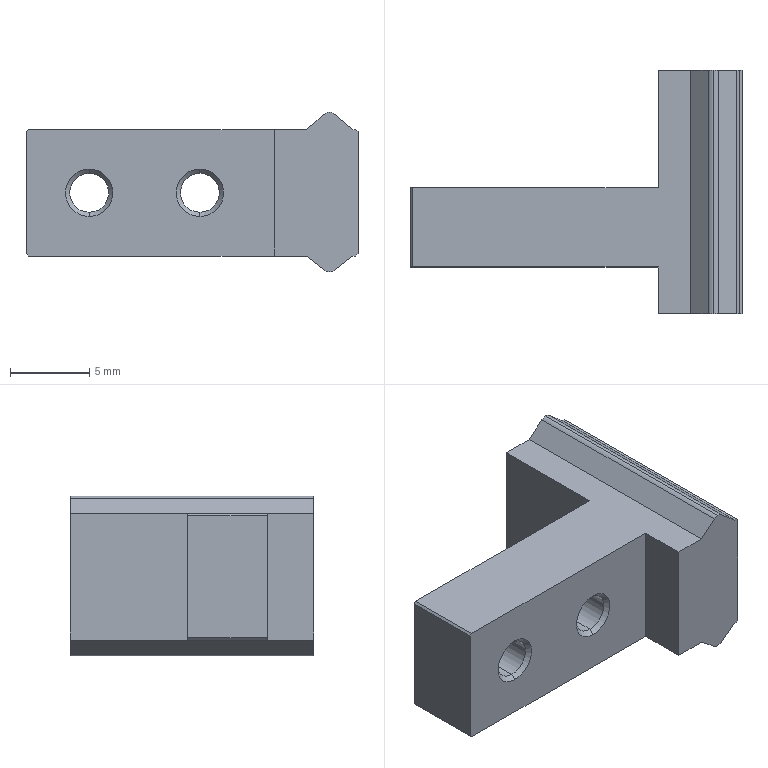Part | SolidWorks | features BaseBody 1 | 1 solid | 35 faces | box 21 x 15.4 x 10.1 mm | volume 1286 mm3 | plane 20 | cone 8 | cylinder 7 | commonest cylinder face diameters 2.459 x4 1 x3
STEP:
#1=CARTESIAN_POINT('',(-48.3,-0.01,5.1));
#2=VERTEX_POINT('',#1);
#3=CARTESIAN_POINT('',(-47.977,-0.01,4.981));
#4=VERTEX_POINT('',#3);
#5=CARTESIAN_POINT('',(-48.3,-0.01,4.6));
#6=DIRECTION('',(0.,1.,0.));
#7=DIRECTION('',(1.,0.,0.));
#8=AXIS2_PLACEMENT_3D('',#5,#6,#7);
#9=CIRCLE('',#8,0.5);
#10=EDGE_CURVE('',#2,#4,#9,.T.);
#11=ORIENTED_EDGE('',*,*,#10,.F.);
#12=CARTESIAN_POINT('',(-48.3,-15.41,5.1));
#13=VERTEX_POINT('',#12);
#14=CARTESIAN_POINT('',(-48.3,-15.41,5.1));
#15=DIRECTION('',(0.,-1.,0.));
#16=VECTOR('',#15,1000.);
#17=LINE('',#14,#16);
#18=EDGE_CURVE('',#2,#13,#17,.T.);
#19=ORIENTED_EDGE('',*,*,#18,.T.);
#20=CARTESIAN_POINT('',(-47.977,-15.41,4.981));
#21=VERTEX_POINT('',#20);
#22=CARTESIAN_POINT('',(-48.3,-15.41,4.6));
#23=DIRECTION('',(0.,1.,0.));
#24=DIRECTION('',(1.,0.,0.));
#25=AXIS2_PLACEMENT_3D('',#22,#23,#24);
#26=CIRCLE('',#25,0.5);
#27=EDGE_CURVE('',#13,#21,#26,.T.);
#28=ORIENTED_EDGE('',*,*,#27,.T.);
#29=CARTESIAN_POINT('',(-47.977,-15.41,4.981));
#30=DIRECTION('',(0.,1.,0.));
#31=VECTOR('',#30,1000.);
#32=LINE('',#29,#31);
#33=EDGE_CURVE('',#21,#4,#32,.T.);
#34=ORIENTED_EDGE('',*,*,#33,.T.);
#35=EDGE_LOOP('',(#11,#19,#28,#34));
#36=FACE_OUTER_BOUND('',#35,.T.);
#37=CARTESIAN_POINT('',(-48.3,-15.41,4.6));
#38=DIRECTION('',(0.,-1.,0.));
#39=DIRECTION('',(0.,0.,1.));
#40=AXIS2_PLACEMENT_3D('',#37,#38,#39);
#41=CYLINDRICAL_SURFACE('',#40,0.5);
#42=ADVANCED_FACE('',(#36),#41,.T.);
#43=CARTESIAN_POINT('',(-63.5,-12.19,-1.229));
#44=VERTEX_POINT('',#43);
#45=CARTESIAN_POINT('',(-63.5,-12.19,1.229));
#46=VERTEX_POINT('',#45);
#47=CARTESIAN_POINT('',(-63.5,-12.19,0.));
#48=DIRECTION('',(0.,1.,0.));
#49=DIRECTION('',(0.,0.,1.));
#50=AXIS2_PLACEMENT_3D('',#47,#48,#49);
#51=CIRCLE('',#50,1.229);
#52=EDGE_CURVE('',#44,#46,#51,.T.);
#53=ORIENTED_EDGE('',*,*,#52,.T.);
#54=CARTESIAN_POINT('',(-63.5,-12.46,1.5));
#55=VERTEX_POINT('',#54);
#56=CARTESIAN_POINT('',(-63.5,-12.46,1.5));
#57=DIRECTION('',(0.,-0.7071,0.7071));
#58=VECTOR('',#57,1000.);
#59=LINE('',#56,#58);
#60=EDGE_CURVE('',#46,#55,#59,.T.);
#61=ORIENTED_EDGE('',*,*,#60,.T.);
#62=CARTESIAN_POINT('',(-63.5,-12.46,-1.5));
#63=VERTEX_POINT('',#62);
#64=CARTESIAN_POINT('',(-63.5,-12.46,0.));
#65=DIRECTION('',(0.,1.,0.));
#66=DIRECTION('',(0.,0.,1.));
#67=AXIS2_PLACEMENT_3D('',#64,#65,#66);
#68=CIRCLE('',#67,1.5);
#69=EDGE_CURVE('',#63,#55,#68,.T.);
#70=ORIENTED_EDGE('',*,*,#69,.F.);
#71=CARTESIAN_POINT('',(-63.5,-12.46,-1.5));
#72=DIRECTION('',(0.,-0.7071,-0.7071));
#73=VECTOR('',#72,1000.);
#74=LINE('',#71,#73);
#75=EDGE_CURVE('',#44,#63,#74,.T.);
#76=ORIENTED_EDGE('',*,*,#75,.F.);
#77=EDGE_LOOP('',(#53,#61,#70,#76));
#78=FACE_OUTER_BOUND('',#77,.T.);
#79=CARTESIAN_POINT('',(-63.5,-12.46,0.));
#80=DIRECTION('',(0.,-1.,0.));
#81=DIRECTION('',(0.,0.,-1.));
#82=AXIS2_PLACEMENT_3D('',#79,#80,#81);
#83=CONICAL_SURFACE('',#82,1.5,0.7854);
#84=ADVANCED_FACE('',(#78),#83,.F.);
#85=CARTESIAN_POINT('',(-63.5,-7.721,1.229));
#86=VERTEX_POINT('',#85);
#87=CARTESIAN_POINT('',(-63.5,-7.721,-1.229));
#88=VERTEX_POINT('',#87);
#89=CARTESIAN_POINT('',(-63.5,-7.721,0.));
#90=DIRECTION('',(0.,1.,0.));
#91=DIRECTION('',(0.,0.,1.));
#92=AXIS2_PLACEMENT_3D('',#89,#90,#91);
#93=CIRCLE('',#92,1.229);
#94=EDGE_CURVE('',#86,#88,#93,.T.);
#95=ORIENTED_EDGE('',*,*,#94,.T.);
#96=CARTESIAN_POINT('',(-63.5,-7.45,-1.229));
#97=DIRECTION('',(0.,-1.,0.));
#98=VECTOR('',#97,1000.);
#99=LINE('',#96,#98);
#100=EDGE_CURVE('',#88,#44,#99,.T.);
#101=ORIENTED_EDGE('',*,*,#100,.T.);
#102=CARTESIAN_POINT('',(-63.5,-12.19,0.));
#103=DIRECTION('',(0.,1.,0.));
#104=DIRECTION('',(0.,0.,1.));
#105=AXIS2_PLACEMENT_3D('',#102,#103,#104);
#106=CIRCLE('',#105,1.229);
#107=EDGE_CURVE('',#46,#44,#106,.T.);
#108=ORIENTED_EDGE('',*,*,#107,.F.);
#109=CARTESIAN_POINT('',(-63.5,-7.45,1.229));
#110=DIRECTION('',(0.,-1.,0.));
#111=VECTOR('',#110,1000.);
#112=LINE('',#109,#111);
#113=EDGE_CURVE('',#86,#46,#112,.T.);
#114=ORIENTED_EDGE('',*,*,#113,.F.);
#115=EDGE_LOOP('',(#95,#101,#108,#114));
#116=FACE_OUTER_BOUND('',#115,.T.);
#117=CARTESIAN_POINT('',(-63.5,-7.45,0.));
#118=DIRECTION('',(0.,-1.,0.));
#119=DIRECTION('',(0.,0.,1.));
#120=AXIS2_PLACEMENT_3D('',#117,#118,#119);
#121=CYLINDRICAL_SURFACE('',#120,1.229);
#122=ADVANCED_FACE('',(#116),#121,.F.);
#123=CARTESIAN_POINT('',(-63.5,-7.721,0.));
#124=DIRECTION('',(0.,1.,0.));
#125=DIRECTION('',(0.,0.,1.));
#126=AXIS2_PLACEMENT_3D('',#123,#124,#125);
#127=CIRCLE('',#126,1.229);
#128=EDGE_CURVE('',#88,#86,#127,.T.);
#129=ORIENTED_EDGE('',*,*,#128,.F.);
#130=CARTESIAN_POINT('',(-63.5,-7.45,-1.5));
#131=VERTEX_POINT('',#130);
#132=CARTESIAN_POINT('',(-63.5,-7.721,-1.229));
#133=DIRECTION('',(0.,0.7071,-0.7071));
#134=VECTOR('',#133,1000.);
#135=LINE('',#132,#134);
#136=EDGE_CURVE('',#88,#131,#135,.T.);
#137=ORIENTED_EDGE('',*,*,#136,.T.);
#138=CARTESIAN_POINT('',(-63.5,-7.45,1.5));
#139=VERTEX_POINT('',#138);
#140=CARTESIAN_POINT('',(-63.5,-7.45,0.));
#141=DIRECTION('',(0.,1.,0.));
#142=DIRECTION('',(0.,0.,1.));
#143=AXIS2_PLACEMENT_3D('',#140,#141,#142);
#144=CIRCLE('',#143,1.5);
#145=EDGE_CURVE('',#131,#139,#144,.T.);
#146=ORIENTED_EDGE('',*,*,#145,.T.);
#147=CARTESIAN_POINT('',(-63.5,-7.721,1.229));
#148=DIRECTION('',(0.,0.7071,0.7071));
#149=VECTOR('',#148,1000.);
#150=LINE('',#147,#149);
#151=EDGE_CURVE('',#86,#139,#150,.T.);
#152=ORIENTED_EDGE('',*,*,#151,.F.);
#153=EDGE_LOOP('',(#129,#137,#146,#152));
#154=FACE_OUTER_BOUND('',#153,.T.);
#155=CARTESIAN_POINT('',(-63.5,-7.721,0.));
#156=DIRECTION('',(0.,1.,0.));
#157=DIRECTION('',(0.,0.,1.));
#158=AXIS2_PLACEMENT_3D('',#155,#156,#157);
#159=CONICAL_SURFACE('',#158,1.229,0.7854);
#160=ADVANCED_FACE('',(#154),#159,.F.);
#161=CARTESIAN_POINT('',(-56.5,-12.19,-1.229));
#162=VERTEX_POINT('',#161);
#163=CARTESIAN_POINT('',(-56.5,-12.19,1.229));
#164=VERTEX_POINT('',#163);
#165=CARTESIAN_POINT('',(-56.5,-12.19,0.));
#166=DIRECTION('',(0.,1.,0.));
#167=DIRECTION('',(0.,0.,1.));
#168=AXIS2_PLACEMENT_3D('',#165,#166,#167);
#169=CIRCLE('',#168,1.229);
#170=EDGE_CURVE('',#162,#164,#169,.T.);
#171=ORIENTED_EDGE('',*,*,#170,.T.);
#172=CARTESIAN_POINT('',(-56.5,-12.46,1.5));
#173=VERTEX_POINT('',#172);
#174=CARTESIAN_POINT('',(-56.5,-12.46,1.5));
#175=DIRECTION('',(0.,-0.7071,0.7071));
#176=VECTOR('',#175,1000.);
#177=LINE('',#174,#176);
#178=EDGE_CURVE('',#164,#173,#177,.T.);
#179=ORIENTED_EDGE('',*,*,#178,.T.);
#180=CARTESIAN_POINT('',(-56.5,-12.46,-1.5));
#181=VERTEX_POINT('',#180);
#182=CARTESIAN_POINT('',(-56.5,-12.46,0.));
#183=DIRECTION('',(0.,1.,0.));
#184=DIRECTION('',(0.,0.,1.));
#185=AXIS2_PLACEMENT_3D('',#182,#183,#184);
#186=CIRCLE('',#185,1.5);
#187=EDGE_CURVE('',#181,#173,#186,.T.);
#188=ORIENTED_EDGE('',*,*,#187,.F.);
#189=CARTESIAN_POINT('',(-56.5,-12.46,-1.5));
#190=DIRECTION('',(0.,-0.7071,-0.7071));
#191=VECTOR('',#190,1000.);
#192=LINE('',#189,#191);
#193=EDGE_CURVE('',#162,#181,#192,.T.);
#194=ORIENTED_EDGE('',*,*,#193,.F.);
#195=EDGE_LOOP('',(#171,#179,#188,#194));
#196=FACE_OUTER_BOUND('',#195,.T.);
#197=CARTESIAN_POINT('',(-56.5,-12.46,0.));
#198=DIRECTION('',(0.,-1.,0.));
#199=DIRECTION('',(0.,0.,-1.));
#200=AXIS2_PLACEMENT_3D('',#197,#198,#199);
#201=CONICAL_SURFACE('',#200,1.5,0.7854);
#202=ADVANCED_FACE('',(#196),#201,.F.);
#203=CARTESIAN_POINT('',(-56.5,-7.721,1.229));
#204=VERTEX_POINT('',#203);
#205=CARTESIAN_POINT('',(-56.5,-7.721,-1.229));
#206=VERTEX_POINT('',#205);
#207=CARTESIAN_POINT('',(-56.5,-7.721,0.));
#208=DIRECTION('',(0.,1.,0.));
#209=DIRECTION('',(0.,0.,1.));
#210=AXIS2_PLACEMENT_3D('',#207,#208,#209);
#211=CIRCLE('',#210,1.229);
#212=EDGE_CURVE('',#204,#206,#211,.T.);
#213=ORIENTED_EDGE('',*,*,#212,.T.);
#214=CARTESIAN_POINT('',(-56.5,-7.45,-1.229));
#215=DIRECTION('',(0.,-1.,0.));
#216=VECTOR('',#215,1000.);
#217=LINE('',#214,#216);
#218=EDGE_CURVE('',#206,#162,#217,.T.);
#219=ORIENTED_EDGE('',*,*,#218,.T.);
#220=CARTESIAN_POINT('',(-56.5,-12.19,0.));
#221=DIRECTION('',(0.,1.,0.));
#222=DIRECTION('',(0.,0.,1.));
#223=AXIS2_PLACEMENT_3D('',#220,#221,#222);
#224=CIRCLE('',#223,1.229);
#225=EDGE_CURVE('',#164,#162,#224,.T.);
#226=ORIENTED_EDGE('',*,*,#225,.F.);
#227=CARTESIAN_POINT('',(-56.5,-7.45,1.229));
#228=DIRECTION('',(0.,-1.,0.));
#229=VECTOR('',#228,1000.);
#230=LINE('',#227,#229);
#231=EDGE_CURVE('',#204,#164,#230,.T.);
#232=ORIENTED_EDGE('',*,*,#231,.F.);
#233=EDGE_LOOP('',(#213,#219,#226,#232));
#234=FACE_OUTER_BOUND('',#233,.T.);
#235=CARTESIAN_POINT('',(-56.5,-7.45,0.));
#236=DIRECTION('',(0.,-1.,0.));
#237=DIRECTION('',(0.,0.,1.));
#238=AXIS2_PLACEMENT_3D('',#235,#236,#237);
#239=CYLINDRICAL_SURFACE('',#238,1.229);
#240=ADVANCED_FACE('',(#234),#239,.F.);
#241=CARTESIAN_POINT('',(-56.5,-7.721,0.));
#242=DIRECTION('',(0.,1.,0.));
#243=DIRECTION('',(0.,0.,1.));
#244=AXIS2_PLACEMENT_3D('',#241,#242,#243);
#245=CIRCLE('',#244,1.229);
#246=EDGE_CURVE('',#206,#204,#245,.T.);
#247=ORIENTED_EDGE('',*,*,#246,.F.);
#248=CARTESIAN_POINT('',(-56.5,-7.45,-1.5));
#249=VERTEX_POINT('',#248);
#250=CARTESIAN_POINT('',(-56.5,-7.721,-1.229));
#251=DIRECTION('',(0.,0.7071,-0.7071));
#252=VECTOR('',#251,1000.);
#253=LINE('',#250,#252);
#254=EDGE_CURVE('',#206,#249,#253,.T.);
#255=ORIENTED_EDGE('',*,*,#254,.T.);
#256=CARTESIAN_POINT('',(-56.5,-7.45,1.5));
#257=VERTEX_POINT('',#256);
#258=CARTESIAN_POINT('',(-56.5,-7.45,0.));
#259=DIRECTION('',(0.,1.,0.));
#260=DIRECTION('',(0.,0.,1.));
#261=AXIS2_PLACEMENT_3D('',#258,#259,#260);
#262=CIRCLE('',#261,1.5);
#263=EDGE_CURVE('',#249,#257,#262,.T.);
#264=ORIENTED_EDGE('',*,*,#263,.T.);
#265=CARTESIAN_POINT('',(-56.5,-7.721,1.229));
#266=DIRECTION('',(0.,0.7071,0.7071));
#267=VECTOR('',#266,1000.);
#268=LINE('',#265,#267);
#269=EDGE_CURVE('',#204,#257,#268,.T.);
#270=ORIENTED_EDGE('',*,*,#269,.F.);
#271=EDGE_LOOP('',(#247,#255,#264,#270));
#272=FACE_OUTER_BOUND('',#271,.T.);
#273=CARTESIAN_POINT('',(-56.5,-7.721,0.));
#274=DIRECTION('',(0.,1.,0.));
#275=DIRECTION('',(0.,0.,1.));
#276=AXIS2_PLACEMENT_3D('',#273,#274,#275);
#277=CONICAL_SURFACE('',#276,1.229,0.7854);
#278=ADVANCED_FACE('',(#272),#277,.F.);
#279=ORIENTED_EDGE('',*,*,#254,.F.);
#280=ORIENTED_EDGE('',*,*,#212,.F.);
#281=ORIENTED_EDGE('',*,*,#269,.T.);
#282=CARTESIAN_POINT('',(-56.5,-7.45,0.));
#283=DIRECTION('',(0.,1.,0.));
#284=DIRECTION('',(0.,0.,1.));
#285=AXIS2_PLACEMENT_3D('',#282,#283,#284);
#286=CIRCLE('',#285,1.5);
#287=EDGE_CURVE('',#257,#249,#286,.T.);
#288=ORIENTED_EDGE('',*,*,#287,.T.);
#289=EDGE_LOOP('',(#279,#280,#281,#288));
#290=FACE_OUTER_BOUND('',#289,.T.);
#291=CARTESIAN_POINT('',(-56.5,-7.721,0.));
#292=DIRECTION('',(0.,1.,0.));
#293=DIRECTION('',(0.,0.,1.));
#294=AXIS2_PLACEMENT_3D('',#291,#292,#293);
#295=CONICAL_SURFACE('',#294,1.229,0.7854);
#296=ADVANCED_FACE('',(#290),#295,.F.);
#297=ORIENTED_EDGE('',*,*,#218,.F.);
#298=ORIENTED_EDGE('',*,*,#246,.T.);
#299=ORIENTED_EDGE('',*,*,#231,.T.);
#300=ORIENTED_EDGE('',*,*,#170,.F.);
#301=EDGE_LOOP('',(#297,#298,#299,#300));
#302=FACE_OUTER_BOUND('',#301,.T.);
#303=CARTESIAN_POINT('',(-56.5,-7.45,0.));
#304=DIRECTION('',(0.,-1.,0.));
#305=DIRECTION('',(0.,0.,1.));
#306=AXIS2_PLACEMENT_3D('',#303,#304,#305);
#307=CYLINDRICAL_SURFACE('',#306,1.229);
#308=ADVANCED_FACE('',(#302),#307,.F.);
#309=ORIENTED_EDGE('',*,*,#178,.F.);
#310=ORIENTED_EDGE('',*,*,#225,.T.);
#311=ORIENTED_EDGE('',*,*,#193,.T.);
#312=CARTESIAN_POINT('',(-56.5,-12.46,0.));
#313=DIRECTION('',(0.,1.,0.));
#314=DIRECTION('',(0.,0.,1.));
#315=AXIS2_PLACEMENT_3D('',#312,#313,#314);
#316=CIRCLE('',#315,1.5);
#317=EDGE_CURVE('',#173,#181,#316,.T.);
#318=ORIENTED_EDGE('',*,*,#317,.F.);
#319=EDGE_LOOP('',(#309,#310,#311,#318));
#320=FACE_OUTER_BOUND('',#319,.T.);
#321=CARTESIAN_POINT('',(-56.5,-12.46,0.));
#322=DIRECTION('',(0.,-1.,0.));
#323=DIRECTION('',(0.,0.,-1.));
#324=AXIS2_PLACEMENT_3D('',#321,#322,#323);
#325=CONICAL_SURFACE('',#324,1.5,0.7854);
#326=ADVANCED_FACE('',(#320),#325,.F.);
#327=ORIENTED_EDGE('',*,*,#136,.F.);
#328=ORIENTED_EDGE('',*,*,#94,.F.);
#329=ORIENTED_EDGE('',*,*,#151,.T.);
#330=CARTESIAN_POINT('',(-63.5,-7.45,0.));
#331=DIRECTION('',(0.,1.,0.));
#332=DIRECTION('',(0.,0.,1.));
#333=AXIS2_PLACEMENT_3D('',#330,#331,#332);
#334=CIRCLE('',#333,1.5);
#335=EDGE_CURVE('',#139,#131,#334,.T.);
#336=ORIENTED_EDGE('',*,*,#335,.T.);
#337=EDGE_LOOP('',(#327,#328,#329,#336));
#338=FACE_OUTER_BOUND('',#337,.T.);
#339=CARTESIAN_POINT('',(-63.5,-7.721,0.));
#340=DIRECTION('',(0.,1.,0.));
#341=DIRECTION('',(0.,0.,1.));
#342=AXIS2_PLACEMENT_3D('',#339,#340,#341);
#343=CONICAL_SURFACE('',#342,1.229,0.7854);
#344=ADVANCED_FACE('',(#338),#343,.F.);
#345=ORIENTED_EDGE('',*,*,#100,.F.);
#346=ORIENTED_EDGE('',*,*,#128,.T.);
#347=ORIENTED_EDGE('',*,*,#113,.T.);
#348=ORIENTED_EDGE('',*,*,#52,.F.);
#349=EDGE_LOOP('',(#345,#346,#347,#348));
#350=FACE_OUTER_BOUND('',#349,.T.);
#351=CARTESIAN_POINT('',(-63.5,-7.45,0.));
#352=DIRECTION('',(0.,-1.,0.));
#353=DIRECTION('',(0.,0.,1.));
#354=AXIS2_PLACEMENT_3D('',#351,#352,#353);
#355=CYLINDRICAL_SURFACE('',#354,1.229);
#356=ADVANCED_FACE('',(#350),#355,.F.);
#357=ORIENTED_EDGE('',*,*,#60,.F.);
#358=ORIENTED_EDGE('',*,*,#107,.T.);
#359=ORIENTED_EDGE('',*,*,#75,.T.);
#360=CARTESIAN_POINT('',(-63.5,-12.46,0.));
#361=DIRECTION('',(0.,1.,0.));
#362=DIRECTION('',(0.,0.,1.));
#363=AXIS2_PLACEMENT_3D('',#360,#361,#362);
#364=CIRCLE('',#363,1.5);
#365=EDGE_CURVE('',#55,#63,#364,.T.);
#366=ORIENTED_EDGE('',*,*,#365,.F.);
#367=EDGE_LOOP('',(#357,#358,#359,#366));
#368=FACE_OUTER_BOUND('',#367,.T.);
#369=CARTESIAN_POINT('',(-63.5,-12.46,0.));
#370=DIRECTION('',(0.,-1.,0.));
#371=DIRECTION('',(0.,0.,-1.));
#372=AXIS2_PLACEMENT_3D('',#369,#370,#371);
#373=CONICAL_SURFACE('',#372,1.5,0.7854);
#374=ADVANCED_FACE('',(#368),#373,.F.);
#375=ORIENTED_EDGE('',*,*,#335,.F.);
#376=ORIENTED_EDGE('',*,*,#145,.F.);
#377=EDGE_LOOP('',(#375,#376));
#378=FACE_BOUND('',#377,.T.);
#379=ORIENTED_EDGE('',*,*,#287,.F.);
#380=ORIENTED_EDGE('',*,*,#263,.F.);
#381=EDGE_LOOP('',(#379,#380));
#382=FACE_BOUND('',#381,.T.);
#383=CARTESIAN_POINT('',(-67.359,-7.45,-4.));
#384=VERTEX_POINT('',#383);
#385=CARTESIAN_POINT('',(-67.5,-7.45,-3.859));
#386=VERTEX_POINT('',#385);
#387=CARTESIAN_POINT('',(-67.359,-7.45,-4.));
#388=DIRECTION('',(-0.7071,0.,0.7071));
#389=VECTOR('',#388,1000.);
#390=LINE('',#387,#389);
#391=EDGE_CURVE('',#384,#386,#390,.T.);
#392=ORIENTED_EDGE('',*,*,#391,.T.);
#393=CARTESIAN_POINT('',(-67.5,-7.45,3.859));
#394=VERTEX_POINT('',#393);
#395=CARTESIAN_POINT('',(-67.5,-7.45,-3.859));
#396=DIRECTION('',(0.,0.,1.));
#397=VECTOR('',#396,1000.);
#398=LINE('',#395,#397);
#399=EDGE_CURVE('',#386,#394,#398,.T.);
#400=ORIENTED_EDGE('',*,*,#399,.T.);
#401=CARTESIAN_POINT('',(-67.359,-7.45,4.));
#402=VERTEX_POINT('',#401);
#403=CARTESIAN_POINT('',(-67.5,-7.45,3.859));
#404=DIRECTION('',(0.7071,0.,0.7071));
#405=VECTOR('',#404,1000.);
#406=LINE('',#403,#405);
#407=EDGE_CURVE('',#394,#402,#406,.T.);
#408=ORIENTED_EDGE('',*,*,#407,.T.);
#409=CARTESIAN_POINT('',(-51.8,-7.45,4.));
#410=VERTEX_POINT('',#409);
#411=CARTESIAN_POINT('',(-67.359,-7.45,4.));
#412=DIRECTION('',(1.,0.,0.));
#413=VECTOR('',#412,1000.);
#414=LINE('',#411,#413);
#415=EDGE_CURVE('',#402,#410,#414,.T.);
#416=ORIENTED_EDGE('',*,*,#415,.T.);
#417=CARTESIAN_POINT('',(-51.8,-7.45,-4.));
#418=VERTEX_POINT('',#417);
#419=CARTESIAN_POINT('',(-51.8,-7.45,4.));
#420=DIRECTION('',(0.,0.,-1.));
#421=VECTOR('',#420,1000.);
#422=LINE('',#419,#421);
#423=EDGE_CURVE('',#410,#418,#422,.T.);
#424=ORIENTED_EDGE('',*,*,#423,.T.);
#425=CARTESIAN_POINT('',(-51.8,-7.45,-4.));
#426=DIRECTION('',(-1.,0.,0.));
#427=VECTOR('',#426,1000.);
#428=LINE('',#425,#427);
#429=EDGE_CURVE('',#418,#384,#428,.T.);
#430=ORIENTED_EDGE('',*,*,#429,.T.);
#431=EDGE_LOOP('',(#392,#400,#408,#416,#424,#430));
#432=FACE_OUTER_BOUND('',#431,.T.);
#433=CARTESIAN_POINT('',(0.,-7.45,0.));
#434=DIRECTION('',(0.,1.,0.));
#435=DIRECTION('',(1.,0.,0.));
#436=AXIS2_PLACEMENT_3D('',#433,#434,#435);
#437=PLANE('',#436);
#438=ADVANCED_FACE('',(#378,#382,#432),#437,.T.);
#439=ORIENTED_EDGE('',*,*,#69,.T.);
#440=ORIENTED_EDGE('',*,*,#365,.T.);
#441=EDGE_LOOP('',(#439,#440));
#442=FACE_BOUND('',#441,.T.);
#443=ORIENTED_EDGE('',*,*,#187,.T.);
#444=ORIENTED_EDGE('',*,*,#317,.T.);
#445=EDGE_LOOP('',(#443,#444));
#446=FACE_BOUND('',#445,.T.);
#447=CARTESIAN_POINT('',(-67.359,-12.46,-4.));
#448=VERTEX_POINT('',#447);
#449=CARTESIAN_POINT('',(-67.5,-12.46,-3.859));
#450=VERTEX_POINT('',#449);
#451=CARTESIAN_POINT('',(-67.359,-12.46,-4.));
#452=DIRECTION('',(-0.7071,0.,0.7071));
#453=VECTOR('',#452,1000.);
#454=LINE('',#451,#453);
#455=EDGE_CURVE('',#448,#450,#454,.T.);
#456=ORIENTED_EDGE('',*,*,#455,.F.);
#457=CARTESIAN_POINT('',(-51.8,-12.46,-4.));
#458=VERTEX_POINT('',#457);
#459=CARTESIAN_POINT('',(-51.8,-12.46,-4.));
#460=DIRECTION('',(-1.,0.,0.));
#461=VECTOR('',#460,1000.);
#462=LINE('',#459,#461);
#463=EDGE_CURVE('',#458,#448,#462,.T.);
#464=ORIENTED_EDGE('',*,*,#463,.F.);
#465=CARTESIAN_POINT('',(-51.8,-12.46,4.));
#466=VERTEX_POINT('',#465);
#467=CARTESIAN_POINT('',(-51.8,-12.46,4.));
#468=DIRECTION('',(0.,0.,-1.));
#469=VECTOR('',#468,1000.);
#470=LINE('',#467,#469);
#471=EDGE_CURVE('',#466,#458,#470,.T.);
#472=ORIENTED_EDGE('',*,*,#471,.F.);
#473=CARTESIAN_POINT('',(-67.359,-12.46,4.));
#474=VERTEX_POINT('',#473);
#475=CARTESIAN_POINT('',(-67.359,-12.46,4.));
#476=DIRECTION('',(1.,0.,0.));
#477=VECTOR('',#476,1000.);
#478=LINE('',#475,#477);
#479=EDGE_CURVE('',#474,#466,#478,.T.);
#480=ORIENTED_EDGE('',*,*,#479,.F.);
#481=CARTESIAN_POINT('',(-67.5,-12.46,3.859));
#482=VERTEX_POINT('',#481);
#483=CARTESIAN_POINT('',(-67.5,-12.46,3.859));
#484=DIRECTION('',(0.7071,0.,0.7071));
#485=VECTOR('',#484,1000.);
#486=LINE('',#483,#485);
#487=EDGE_CURVE('',#482,#474,#486,.T.);
#488=ORIENTED_EDGE('',*,*,#487,.F.);
#489=CARTESIAN_POINT('',(-67.5,-12.46,-3.859));
#490=DIRECTION('',(0.,0.,1.));
#491=VECTOR('',#490,1000.);
#492=LINE('',#489,#491);
#493=EDGE_CURVE('',#450,#482,#492,.T.);
#494=ORIENTED_EDGE('',*,*,#493,.F.);
#495=EDGE_LOOP('',(#456,#464,#472,#480,#488,#494));
#496=FACE_OUTER_BOUND('',#495,.T.);
#497=CARTESIAN_POINT('',(0.,-12.46,0.));
#498=DIRECTION('',(0.,1.,0.));
#499=DIRECTION('',(1.,0.,0.));
#500=AXIS2_PLACEMENT_3D('',#497,#498,#499);
#501=PLANE('',#500);
#502=ADVANCED_FACE('',(#442,#446,#496),#501,.F.);
#503=ORIENTED_EDGE('',*,*,#487,.T.);
#504=CARTESIAN_POINT('',(-67.359,-7.45,4.));
#505=DIRECTION('',(0.,-1.,0.));
#506=VECTOR('',#505,1000.);
#507=LINE('',#504,#506);
#508=EDGE_CURVE('',#402,#474,#507,.T.);
#509=ORIENTED_EDGE('',*,*,#508,.F.);
#510=ORIENTED_EDGE('',*,*,#407,.F.);
#511=CARTESIAN_POINT('',(-67.5,-7.45,3.859));
#512=DIRECTION('',(0.,-1.,0.));
#513=VECTOR('',#512,1000.);
#514=LINE('',#511,#513);
#515=EDGE_CURVE('',#394,#482,#514,.T.);
#516=ORIENTED_EDGE('',*,*,#515,.T.);
#517=EDGE_LOOP('',(#503,#509,#510,#516));
#518=FACE_OUTER_BOUND('',#517,.T.);
#519=CARTESIAN_POINT('',(-67.5,-7.45,3.859));
#520=DIRECTION('',(0.7071,0.,-0.7071));
#521=DIRECTION('',(0.,-1.,0.));
#522=AXIS2_PLACEMENT_3D('',#519,#520,#521);
#523=PLANE('',#522);
#524=ADVANCED_FACE('',(#518),#523,.F.);
#525=ORIENTED_EDGE('',*,*,#493,.T.);
#526=ORIENTED_EDGE('',*,*,#515,.F.);
#527=ORIENTED_EDGE('',*,*,#399,.F.);
#528=CARTESIAN_POINT('',(-67.5,-7.45,-3.859));
#529=DIRECTION('',(0.,-1.,0.));
#530=VECTOR('',#529,1000.);
#531=LINE('',#528,#530);
#532=EDGE_CURVE('',#386,#450,#531,.T.);
#533=ORIENTED_EDGE('',*,*,#532,.T.);
#534=EDGE_LOOP('',(#525,#526,#527,#533));
#535=FACE_OUTER_BOUND('',#534,.T.);
#536=CARTESIAN_POINT('',(-67.5,-7.45,-3.859));
#537=DIRECTION('',(1.,0.,0.));
#538=DIRECTION('',(0.,1.,0.));
#539=AXIS2_PLACEMENT_3D('',#536,#537,#538);
#540=PLANE('',#539);
#541=ADVANCED_FACE('',(#535),#540,.F.);
#542=ORIENTED_EDGE('',*,*,#455,.T.);
#543=ORIENTED_EDGE('',*,*,#532,.F.);
#544=ORIENTED_EDGE('',*,*,#391,.F.);
#545=CARTESIAN_POINT('',(-67.359,-7.45,-4.));
#546=DIRECTION('',(0.,-1.,0.));
#547=VECTOR('',#546,1000.);
#548=LINE('',#545,#547);
#549=EDGE_CURVE('',#384,#448,#548,.T.);
#550=ORIENTED_EDGE('',*,*,#549,.T.);
#551=EDGE_LOOP('',(#542,#543,#544,#550));
#552=FACE_OUTER_BOUND('',#551,.T.);
#553=CARTESIAN_POINT('',(-67.359,-7.45,-4.));
#554=DIRECTION('',(0.7071,0.,0.7071));
#555=DIRECTION('',(0.,-1.,0.));
#556=AXIS2_PLACEMENT_3D('',#553,#554,#555);
#557=PLANE('',#556);
#558=ADVANCED_FACE('',(#552),#557,.F.);
#559=CARTESIAN_POINT('',(-51.8,-15.41,-4.));
#560=VERTEX_POINT('',#559);
#561=CARTESIAN_POINT('',(-51.8,-15.41,4.));
#562=VERTEX_POINT('',#561);
#563=CARTESIAN_POINT('',(-51.8,-15.41,-4.));
#564=DIRECTION('',(0.,0.,1.));
#565=VECTOR('',#564,1000.);
#566=LINE('',#563,#565);
#567=EDGE_CURVE('',#560,#562,#566,.T.);
#568=ORIENTED_EDGE('',*,*,#567,.F.);
#569=CARTESIAN_POINT('',(-49.76,-15.41,-4.));
#570=VERTEX_POINT('',#569);
#571=CARTESIAN_POINT('',(-49.76,-15.41,-4.));
#572=DIRECTION('',(-1.,0.,0.));
#573=VECTOR('',#572,1000.);
#574=LINE('',#571,#573);
#575=EDGE_CURVE('',#570,#560,#574,.T.);
#576=ORIENTED_EDGE('',*,*,#575,.F.);
#577=CARTESIAN_POINT('',(-48.607,-15.41,-4.895));
#578=VERTEX_POINT('',#577);
#579=CARTESIAN_POINT('',(-48.607,-15.41,-4.895));
#580=DIRECTION('',(-0.7901,0.,0.613));
#581=VECTOR('',#580,1000.);
#582=LINE('',#579,#581);
#583=EDGE_CURVE('',#578,#570,#582,.T.);
#584=ORIENTED_EDGE('',*,*,#583,.F.);
#585=CARTESIAN_POINT('',(-47.997,-15.41,-4.898));
#586=VERTEX_POINT('',#585);
#587=CARTESIAN_POINT('',(-48.3,-15.41,-4.5));
#588=DIRECTION('',(0.,1.,0.));
#589=DIRECTION('',(1.,0.,0.));
#590=AXIS2_PLACEMENT_3D('',#587,#588,#589);
#591=CIRCLE('',#590,0.5);
#592=EDGE_CURVE('',#586,#578,#591,.T.);
#593=ORIENTED_EDGE('',*,*,#592,.F.);
#594=CARTESIAN_POINT('',(-46.82,-15.41,-4.));
#595=VERTEX_POINT('',#594);
#596=CARTESIAN_POINT('',(-46.82,-15.41,-4.));
#597=DIRECTION('',(-0.7951,0.,-0.6065));
#598=VECTOR('',#597,1000.);
#599=LINE('',#596,#598);
#600=EDGE_CURVE('',#595,#586,#599,.T.);
#601=ORIENTED_EDGE('',*,*,#600,.F.);
#602=CARTESIAN_POINT('',(-46.641,-15.41,-4.));
#603=VERTEX_POINT('',#602);
#604=CARTESIAN_POINT('',(-46.641,-15.41,-4.));
#605=DIRECTION('',(-1.,0.,0.));
#606=VECTOR('',#605,1000.);
#607=LINE('',#604,#606);
#608=EDGE_CURVE('',#603,#595,#607,.T.);
#609=ORIENTED_EDGE('',*,*,#608,.F.);
#610=CARTESIAN_POINT('',(-46.5,-15.41,-3.859));
#611=VERTEX_POINT('',#610);
#612=CARTESIAN_POINT('',(-46.5,-15.41,-3.859));
#613=DIRECTION('',(-0.7071,0.,-0.7071));
#614=VECTOR('',#613,1000.);
#615=LINE('',#612,#614);
#616=EDGE_CURVE('',#611,#603,#615,.T.);
#617=ORIENTED_EDGE('',*,*,#616,.F.);
#618=CARTESIAN_POINT('',(-46.5,-15.41,3.859));
#619=VERTEX_POINT('',#618);
#620=CARTESIAN_POINT('',(-46.5,-15.41,3.859));
#621=DIRECTION('',(0.,0.,-1.));
#622=VECTOR('',#621,1000.);
#623=LINE('',#620,#622);
#624=EDGE_CURVE('',#619,#611,#623,.T.);
#625=ORIENTED_EDGE('',*,*,#624,.F.);
#626=CARTESIAN_POINT('',(-46.641,-15.41,4.));
#627=VERTEX_POINT('',#626);
#628=CARTESIAN_POINT('',(-46.641,-15.41,4.));
#629=DIRECTION('',(0.7071,0.,-0.7071));
#630=VECTOR('',#629,1000.);
#631=LINE('',#628,#630);
#632=EDGE_CURVE('',#627,#619,#631,.T.);
#633=ORIENTED_EDGE('',*,*,#632,.F.);
#634=CARTESIAN_POINT('',(-46.82,-15.41,4.));
#635=VERTEX_POINT('',#634);
#636=CARTESIAN_POINT('',(-46.82,-15.41,4.));
#637=DIRECTION('',(1.,0.,0.));
#638=VECTOR('',#637,1000.);
#639=LINE('',#636,#638);
#640=EDGE_CURVE('',#635,#627,#639,.T.);
#641=ORIENTED_EDGE('',*,*,#640,.F.);
#642=CARTESIAN_POINT('',(-47.977,-15.41,4.981));
#643=DIRECTION('',(0.7625,0.,-0.647));
#644=VECTOR('',#643,1000.);
#645=LINE('',#642,#644);
#646=EDGE_CURVE('',#21,#635,#645,.T.);
#647=ORIENTED_EDGE('',*,*,#646,.F.);
#648=ORIENTED_EDGE('',*,*,#27,.F.);
#649=CARTESIAN_POINT('',(-48.627,-15.41,4.978));
#650=VERTEX_POINT('',#649);
#651=CARTESIAN_POINT('',(-48.3,-15.41,4.6));
#652=DIRECTION('',(0.,1.,0.));
#653=DIRECTION('',(1.,0.,0.));
#654=AXIS2_PLACEMENT_3D('',#651,#652,#653);
#655=CIRCLE('',#654,0.5);
#656=EDGE_CURVE('',#650,#13,#655,.T.);
#657=ORIENTED_EDGE('',*,*,#656,.F.);
#658=CARTESIAN_POINT('',(-49.76,-15.41,4.));
#659=VERTEX_POINT('',#658);
#660=CARTESIAN_POINT('',(-49.76,-15.41,4.));
#661=DIRECTION('',(0.7569,0.,0.6535));
#662=VECTOR('',#661,1000.);
#663=LINE('',#660,#662);
#664=EDGE_CURVE('',#659,#650,#663,.T.);
#665=ORIENTED_EDGE('',*,*,#664,.F.);
#666=CARTESIAN_POINT('',(-51.8,-15.41,4.));
#667=DIRECTION('',(1.,0.,0.));
#668=VECTOR('',#667,1000.);
#669=LINE('',#666,#668);
#670=EDGE_CURVE('',#562,#659,#669,.T.);
#671=ORIENTED_EDGE('',*,*,#670,.F.);
#672=EDGE_LOOP('',(#568,#576,#584,#593,#601,#609,#617,#625,#633,#641,#647,#648,#657,#665,#671));
#673=FACE_OUTER_BOUND('',#672,.T.);
#674=CARTESIAN_POINT('',(-48.3,-15.41,4.6));
#675=DIRECTION('',(0.,1.,0.));
#676=DIRECTION('',(1.,0.,0.));
#677=AXIS2_PLACEMENT_3D('',#674,#675,#676);
#678=PLANE('',#677);
#679=ADVANCED_FACE('',(#673),#678,.F.);
#680=CARTESIAN_POINT('',(-51.8,-0.01,-4.));
#681=VERTEX_POINT('',#680);
#682=CARTESIAN_POINT('',(-51.8,-0.01,4.));
#683=VERTEX_POINT('',#682);
#684=CARTESIAN_POINT('',(-51.8,-0.01,-4.));
#685=DIRECTION('',(0.,0.,1.));
#686=VECTOR('',#685,1000.);
#687=LINE('',#684,#686);
#688=EDGE_CURVE('',#681,#683,#687,.T.);
#689=ORIENTED_EDGE('',*,*,#688,.T.);
#690=CARTESIAN_POINT('',(-49.76,-0.01,4.));
#691=VERTEX_POINT('',#690);
#692=CARTESIAN_POINT('',(-51.8,-0.01,4.));
#693=DIRECTION('',(1.,0.,0.));
#694=VECTOR('',#693,1000.);
#695=LINE('',#692,#694);
#696=EDGE_CURVE('',#683,#691,#695,.T.);
#697=ORIENTED_EDGE('',*,*,#696,.T.);
#698=CARTESIAN_POINT('',(-48.627,-0.01,4.978));
#699=VERTEX_POINT('',#698);
#700=CARTESIAN_POINT('',(-49.76,-0.01,4.));
#701=DIRECTION('',(0.7569,0.,0.6535));
#702=VECTOR('',#701,1000.);
#703=LINE('',#700,#702);
#704=EDGE_CURVE('',#691,#699,#703,.T.);
#705=ORIENTED_EDGE('',*,*,#704,.T.);
#706=CARTESIAN_POINT('',(-48.3,-0.01,4.6));
#707=DIRECTION('',(0.,1.,0.));
#708=DIRECTION('',(1.,0.,0.));
#709=AXIS2_PLACEMENT_3D('',#706,#707,#708);
#710=CIRCLE('',#709,0.5);
#711=EDGE_CURVE('',#699,#2,#710,.T.);
#712=ORIENTED_EDGE('',*,*,#711,.T.);
#713=ORIENTED_EDGE('',*,*,#10,.T.);
#714=CARTESIAN_POINT('',(-46.82,-0.01,4.));
#715=VERTEX_POINT('',#714);
#716=CARTESIAN_POINT('',(-47.977,-0.01,4.981));
#717=DIRECTION('',(0.7625,0.,-0.647));
#718=VECTOR('',#717,1000.);
#719=LINE('',#716,#718);
#720=EDGE_CURVE('',#4,#715,#719,.T.);
#721=ORIENTED_EDGE('',*,*,#720,.T.);
#722=CARTESIAN_POINT('',(-46.641,-0.01,4.));
#723=VERTEX_POINT('',#722);
#724=CARTESIAN_POINT('',(-46.82,-0.01,4.));
#725=DIRECTION('',(1.,0.,0.));
#726=VECTOR('',#725,1000.);
#727=LINE('',#724,#726);
#728=EDGE_CURVE('',#715,#723,#727,.T.);
#729=ORIENTED_EDGE('',*,*,#728,.T.);
#730=CARTESIAN_POINT('',(-46.5,-0.01,3.859));
#731=VERTEX_POINT('',#730);
#732=CARTESIAN_POINT('',(-46.641,-0.01,4.));
#733=DIRECTION('',(0.7071,0.,-0.7071));
#734=VECTOR('',#733,1000.);
#735=LINE('',#732,#734);
#736=EDGE_CURVE('',#723,#731,#735,.T.);
#737=ORIENTED_EDGE('',*,*,#736,.T.);
#738=CARTESIAN_POINT('',(-46.5,-0.01,-3.859));
#739=VERTEX_POINT('',#738);
#740=CARTESIAN_POINT('',(-46.5,-0.01,3.859));
#741=DIRECTION('',(0.,0.,-1.));
#742=VECTOR('',#741,1000.);
#743=LINE('',#740,#742);
#744=EDGE_CURVE('',#731,#739,#743,.T.);
#745=ORIENTED_EDGE('',*,*,#744,.T.);
#746=CARTESIAN_POINT('',(-46.641,-0.01,-4.));
#747=VERTEX_POINT('',#746);
#748=CARTESIAN_POINT('',(-46.5,-0.01,-3.859));
#749=DIRECTION('',(-0.7071,0.,-0.7071));
#750=VECTOR('',#749,1000.);
#751=LINE('',#748,#750);
#752=EDGE_CURVE('',#739,#747,#751,.T.);
#753=ORIENTED_EDGE('',*,*,#752,.T.);
#754=CARTESIAN_POINT('',(-46.82,-0.01,-4.));
#755=VERTEX_POINT('',#754);
#756=CARTESIAN_POINT('',(-46.641,-0.01,-4.));
#757=DIRECTION('',(-1.,0.,0.));
#758=VECTOR('',#757,1000.);
#759=LINE('',#756,#758);
#760=EDGE_CURVE('',#747,#755,#759,.T.);
#761=ORIENTED_EDGE('',*,*,#760,.T.);
#762=CARTESIAN_POINT('',(-47.997,-0.01,-4.898));
#763=VERTEX_POINT('',#762);
#764=CARTESIAN_POINT('',(-46.82,-0.01,-4.));
#765=DIRECTION('',(-0.7951,0.,-0.6065));
#766=VECTOR('',#765,1000.);
#767=LINE('',#764,#766);
#768=EDGE_CURVE('',#755,#763,#767,.T.);
#769=ORIENTED_EDGE('',*,*,#768,.T.);
#770=CARTESIAN_POINT('',(-48.607,-0.01,-4.895));
#771=VERTEX_POINT('',#770);
#772=CARTESIAN_POINT('',(-48.3,-0.01,-4.5));
#773=DIRECTION('',(0.,1.,0.));
#774=DIRECTION('',(1.,0.,0.));
#775=AXIS2_PLACEMENT_3D('',#772,#773,#774);
#776=CIRCLE('',#775,0.5);
#777=EDGE_CURVE('',#763,#771,#776,.T.);
#778=ORIENTED_EDGE('',*,*,#777,.T.);
#779=CARTESIAN_POINT('',(-49.76,-0.01,-4.));
#780=VERTEX_POINT('',#779);
#781=CARTESIAN_POINT('',(-48.607,-0.01,-4.895));
#782=DIRECTION('',(-0.7901,0.,0.613));
#783=VECTOR('',#782,1000.);
#784=LINE('',#781,#783);
#785=EDGE_CURVE('',#771,#780,#784,.T.);
#786=ORIENTED_EDGE('',*,*,#785,.T.);
#787=CARTESIAN_POINT('',(-49.76,-0.01,-4.));
#788=DIRECTION('',(-1.,0.,0.));
#789=VECTOR('',#788,1000.);
#790=LINE('',#787,#789);
#791=EDGE_CURVE('',#780,#681,#790,.T.);
#792=ORIENTED_EDGE('',*,*,#791,.T.);
#793=EDGE_LOOP('',(#689,#697,#705,#712,#713,#721,#729,#737,#745,#753,#761,#769,#778,#786,#792));
#794=FACE_OUTER_BOUND('',#793,.T.);
#795=CARTESIAN_POINT('',(-48.3,-0.01,4.6));
#796=DIRECTION('',(0.,1.,0.));
#797=DIRECTION('',(1.,0.,0.));
#798=AXIS2_PLACEMENT_3D('',#795,#796,#797);
#799=PLANE('',#798);
#800=ADVANCED_FACE('',(#794),#799,.T.);
#801=ORIENTED_EDGE('',*,*,#768,.F.);
#802=CARTESIAN_POINT('',(-46.82,-15.41,-4.));
#803=DIRECTION('',(0.,1.,0.));
#804=VECTOR('',#803,1000.);
#805=LINE('',#802,#804);
#806=EDGE_CURVE('',#595,#755,#805,.T.);
#807=ORIENTED_EDGE('',*,*,#806,.F.);
#808=ORIENTED_EDGE('',*,*,#600,.T.);
#809=CARTESIAN_POINT('',(-47.997,-15.41,-4.898));
#810=DIRECTION('',(0.,1.,0.));
#811=VECTOR('',#810,1000.);
#812=LINE('',#809,#811);
#813=EDGE_CURVE('',#586,#763,#812,.T.);
#814=ORIENTED_EDGE('',*,*,#813,.T.);
#815=EDGE_LOOP('',(#801,#807,#808,#814));
#816=FACE_OUTER_BOUND('',#815,.T.);
#817=CARTESIAN_POINT('',(-46.82,-15.41,-4.));
#818=DIRECTION('',(0.6065,0.,-0.7951));
#819=DIRECTION('',(0.,-1.,0.));
#820=AXIS2_PLACEMENT_3D('',#817,#818,#819);
#821=PLANE('',#820);
#822=ADVANCED_FACE('',(#816),#821,.T.);
#823=ORIENTED_EDGE('',*,*,#760,.F.);
#824=CARTESIAN_POINT('',(-46.641,-15.41,-4.));
#825=DIRECTION('',(0.,1.,0.));
#826=VECTOR('',#825,1000.);
#827=LINE('',#824,#826);
#828=EDGE_CURVE('',#603,#747,#827,.T.);
#829=ORIENTED_EDGE('',*,*,#828,.F.);
#830=ORIENTED_EDGE('',*,*,#608,.T.);
#831=ORIENTED_EDGE('',*,*,#806,.T.);
#832=EDGE_LOOP('',(#823,#829,#830,#831));
#833=FACE_OUTER_BOUND('',#832,.T.);
#834=CARTESIAN_POINT('',(-46.641,-15.41,-4.));
#835=DIRECTION('',(0.,0.,-1.));
#836=DIRECTION('',(0.,-1.,0.));
#837=AXIS2_PLACEMENT_3D('',#834,#835,#836);
#838=PLANE('',#837);
#839=ADVANCED_FACE('',(#833),#838,.T.);
#840=ORIENTED_EDGE('',*,*,#752,.F.);
#841=CARTESIAN_POINT('',(-46.5,-15.41,-3.859));
#842=DIRECTION('',(0.,1.,0.));
#843=VECTOR('',#842,1000.);
#844=LINE('',#841,#843);
#845=EDGE_CURVE('',#611,#739,#844,.T.);
#846=ORIENTED_EDGE('',*,*,#845,.F.);
#847=ORIENTED_EDGE('',*,*,#616,.T.);
#848=ORIENTED_EDGE('',*,*,#828,.T.);
#849=EDGE_LOOP('',(#840,#846,#847,#848));
#850=FACE_OUTER_BOUND('',#849,.T.);
#851=CARTESIAN_POINT('',(-46.5,-15.41,-3.859));
#852=DIRECTION('',(0.7071,0.,-0.7071));
#853=DIRECTION('',(0.,-1.,0.));
#854=AXIS2_PLACEMENT_3D('',#851,#852,#853);
#855=PLANE('',#854);
#856=ADVANCED_FACE('',(#850),#855,.T.);
#857=ORIENTED_EDGE('',*,*,#744,.F.);
#858=CARTESIAN_POINT('',(-46.5,-15.41,3.859));
#859=DIRECTION('',(0.,1.,0.));
#860=VECTOR('',#859,1000.);
#861=LINE('',#858,#860);
#862=EDGE_CURVE('',#619,#731,#861,.T.);
#863=ORIENTED_EDGE('',*,*,#862,.F.);
#864=ORIENTED_EDGE('',*,*,#624,.T.);
#865=ORIENTED_EDGE('',*,*,#845,.T.);
#866=EDGE_LOOP('',(#857,#863,#864,#865));
#867=FACE_OUTER_BOUND('',#866,.T.);
#868=CARTESIAN_POINT('',(-46.5,-15.41,3.859));
#869=DIRECTION('',(1.,0.,0.));
#870=DIRECTION('',(0.,1.,0.));
#871=AXIS2_PLACEMENT_3D('',#868,#869,#870);
#872=PLANE('',#871);
#873=ADVANCED_FACE('',(#867),#872,.T.);
#874=ORIENTED_EDGE('',*,*,#736,.F.);
#875=CARTESIAN_POINT('',(-46.641,-15.41,4.));
#876=DIRECTION('',(0.,1.,0.));
#877=VECTOR('',#876,1000.);
#878=LINE('',#875,#877);
#879=EDGE_CURVE('',#627,#723,#878,.T.);
#880=ORIENTED_EDGE('',*,*,#879,.F.);
#881=ORIENTED_EDGE('',*,*,#632,.T.);
#882=ORIENTED_EDGE('',*,*,#862,.T.);
#883=EDGE_LOOP('',(#874,#880,#881,#882));
#884=FACE_OUTER_BOUND('',#883,.T.);
#885=CARTESIAN_POINT('',(-46.641,-15.41,4.));
#886=DIRECTION('',(0.7071,0.,0.7071));
#887=DIRECTION('',(0.,-1.,0.));
#888=AXIS2_PLACEMENT_3D('',#885,#886,#887);
#889=PLANE('',#888);
#890=ADVANCED_FACE('',(#884),#889,.T.);
#891=ORIENTED_EDGE('',*,*,#728,.F.);
#892=CARTESIAN_POINT('',(-46.82,-15.41,4.));
#893=DIRECTION('',(0.,1.,0.));
#894=VECTOR('',#893,1000.);
#895=LINE('',#892,#894);
#896=EDGE_CURVE('',#635,#715,#895,.T.);
#897=ORIENTED_EDGE('',*,*,#896,.F.);
#898=ORIENTED_EDGE('',*,*,#640,.T.);
#899=ORIENTED_EDGE('',*,*,#879,.T.);
#900=EDGE_LOOP('',(#891,#897,#898,#899));
#901=FACE_OUTER_BOUND('',#900,.T.);
#902=CARTESIAN_POINT('',(-46.82,-15.41,4.));
#903=DIRECTION('',(0.,0.,1.));
#904=DIRECTION('',(1.,0.,0.));
#905=AXIS2_PLACEMENT_3D('',#902,#903,#904);
#906=PLANE('',#905);
#907=ADVANCED_FACE('',(#901),#906,.T.);
#908=ORIENTED_EDGE('',*,*,#720,.F.);
#909=ORIENTED_EDGE('',*,*,#33,.F.);
#910=ORIENTED_EDGE('',*,*,#646,.T.);
#911=ORIENTED_EDGE('',*,*,#896,.T.);
#912=EDGE_LOOP('',(#908,#909,#910,#911));
#913=FACE_OUTER_BOUND('',#912,.T.);
#914=CARTESIAN_POINT('',(-47.977,-15.41,4.981));
#915=DIRECTION('',(0.647,0.,0.7625));
#916=DIRECTION('',(0.,-1.,0.));
#917=AXIS2_PLACEMENT_3D('',#914,#915,#916);
#918=PLANE('',#917);
#919=ADVANCED_FACE('',(#913),#918,.T.);
#920=ORIENTED_EDGE('',*,*,#18,.F.);
#921=ORIENTED_EDGE('',*,*,#711,.F.);
#922=CARTESIAN_POINT('',(-48.627,-15.41,4.978));
#923=DIRECTION('',(0.,1.,0.));
#924=VECTOR('',#923,1000.);
#925=LINE('',#922,#924);
#926=EDGE_CURVE('',#650,#699,#925,.T.);
#927=ORIENTED_EDGE('',*,*,#926,.F.);
#928=ORIENTED_EDGE('',*,*,#656,.T.);
#929=EDGE_LOOP('',(#920,#921,#927,#928));
#930=FACE_OUTER_BOUND('',#929,.T.);
#931=CARTESIAN_POINT('',(-48.3,-15.41,4.6));
#932=DIRECTION('',(0.,-1.,0.));
#933=DIRECTION('',(0.,0.,1.));
#934=AXIS2_PLACEMENT_3D('',#931,#932,#933);
#935=CYLINDRICAL_SURFACE('',#934,0.5);
#936=ADVANCED_FACE('',(#930),#935,.T.);
#937=ORIENTED_EDGE('',*,*,#704,.F.);
#938=CARTESIAN_POINT('',(-49.76,-15.41,4.));
#939=DIRECTION('',(0.,1.,0.));
#940=VECTOR('',#939,1000.);
#941=LINE('',#938,#940);
#942=EDGE_CURVE('',#659,#691,#941,.T.);
#943=ORIENTED_EDGE('',*,*,#942,.F.);
#944=ORIENTED_EDGE('',*,*,#664,.T.);
#945=ORIENTED_EDGE('',*,*,#926,.T.);
#946=EDGE_LOOP('',(#937,#943,#944,#945));
#947=FACE_OUTER_BOUND('',#946,.T.);
#948=CARTESIAN_POINT('',(-49.76,-15.41,4.));
#949=DIRECTION('',(-0.6535,0.,0.7569));
#950=DIRECTION('',(0.,1.,0.));
#951=AXIS2_PLACEMENT_3D('',#948,#949,#950);
#952=PLANE('',#951);
#953=ADVANCED_FACE('',(#947),#952,.T.);
#954=ORIENTED_EDGE('',*,*,#696,.F.);
#955=CARTESIAN_POINT('',(-51.8,-15.41,4.));
#956=DIRECTION('',(0.,1.,0.));
#957=VECTOR('',#956,1000.);
#958=LINE('',#955,#957);
#959=EDGE_CURVE('',#410,#683,#958,.T.);
#960=ORIENTED_EDGE('',*,*,#959,.F.);
#961=ORIENTED_EDGE('',*,*,#415,.F.);
#962=ORIENTED_EDGE('',*,*,#508,.T.);
#963=ORIENTED_EDGE('',*,*,#479,.T.);
#964=CARTESIAN_POINT('',(-51.8,-15.41,4.));
#965=DIRECTION('',(0.,1.,0.));
#966=VECTOR('',#965,1000.);
#967=LINE('',#964,#966);
#968=EDGE_CURVE('',#562,#466,#967,.T.);
#969=ORIENTED_EDGE('',*,*,#968,.F.);
#970=ORIENTED_EDGE('',*,*,#670,.T.);
#971=ORIENTED_EDGE('',*,*,#942,.T.);
#972=EDGE_LOOP('',(#954,#960,#961,#962,#963,#969,#970,#971));
#973=FACE_OUTER_BOUND('',#972,.T.);
#974=CARTESIAN_POINT('',(-51.8,-15.41,4.));
#975=DIRECTION('',(0.,0.,1.));
#976=DIRECTION('',(1.,0.,0.));
#977=AXIS2_PLACEMENT_3D('',#974,#975,#976);
#978=PLANE('',#977);
#979=ADVANCED_FACE('',(#973),#978,.T.);
#980=ORIENTED_EDGE('',*,*,#423,.F.);
#981=ORIENTED_EDGE('',*,*,#959,.T.);
#982=ORIENTED_EDGE('',*,*,#688,.F.);
#983=CARTESIAN_POINT('',(-51.8,-15.41,-4.));
#984=DIRECTION('',(0.,1.,0.));
#985=VECTOR('',#984,1000.);
#986=LINE('',#983,#985);
#987=EDGE_CURVE('',#418,#681,#986,.T.);
#988=ORIENTED_EDGE('',*,*,#987,.F.);
#989=EDGE_LOOP('',(#980,#981,#982,#988));
#990=FACE_OUTER_BOUND('',#989,.T.);
#991=CARTESIAN_POINT('',(-51.8,-15.41,-4.));
#992=DIRECTION('',(-1.,0.,0.));
#993=DIRECTION('',(0.,0.,1.));
#994=AXIS2_PLACEMENT_3D('',#991,#992,#993);
#995=PLANE('',#994);
#996=ADVANCED_FACE('',(#990),#995,.T.);
#997=ORIENTED_EDGE('',*,*,#968,.T.);
#998=ORIENTED_EDGE('',*,*,#471,.T.);
#999=CARTESIAN_POINT('',(-51.8,-15.41,-4.));
#1000=DIRECTION('',(0.,1.,0.));
#1001=VECTOR('',#1000,1000.);
#1002=LINE('',#999,#1001);
#1003=EDGE_CURVE('',#560,#458,#1002,.T.);
#1004=ORIENTED_EDGE('',*,*,#1003,.F.);
#1005=ORIENTED_EDGE('',*,*,#567,.T.);
#1006=EDGE_LOOP('',(#997,#998,#1004,#1005));
#1007=FACE_OUTER_BOUND('',#1006,.T.);
#1008=CARTESIAN_POINT('',(-51.8,-15.41,-4.));
#1009=DIRECTION('',(-1.,0.,0.));
#1010=DIRECTION('',(0.,0.,1.));
#1011=AXIS2_PLACEMENT_3D('',#1008,#1009,#1010);
#1012=PLANE('',#1011);
#1013=ADVANCED_FACE('',(#1007),#1012,.T.);
#1014=ORIENTED_EDGE('',*,*,#777,.F.);
#1015=ORIENTED_EDGE('',*,*,#813,.F.);
#1016=ORIENTED_EDGE('',*,*,#592,.T.);
#1017=CARTESIAN_POINT('',(-48.607,-15.41,-4.895));
#1018=DIRECTION('',(0.,1.,0.));
#1019=VECTOR('',#1018,1000.);
#1020=LINE('',#1017,#1019);
#1021=EDGE_CURVE('',#578,#771,#1020,.T.);
#1022=ORIENTED_EDGE('',*,*,#1021,.T.);
#1023=EDGE_LOOP('',(#1014,#1015,#1016,#1022));
#1024=FACE_OUTER_BOUND('',#1023,.T.);
#1025=CARTESIAN_POINT('',(-48.3,-15.41,-4.5));
#1026=DIRECTION('',(0.,-1.,0.));
#1027=DIRECTION('',(0.,0.,1.));
#1028=AXIS2_PLACEMENT_3D('',#1025,#1026,#1027);
#1029=CYLINDRICAL_SURFACE('',#1028,0.5);
#1030=ADVANCED_FACE('',(#1024),#1029,.T.);
#1031=ORIENTED_EDGE('',*,*,#791,.F.);
#1032=CARTESIAN_POINT('',(-49.76,-15.41,-4.));
#1033=DIRECTION('',(0.,1.,0.));
#1034=VECTOR('',#1033,1000.);
#1035=LINE('',#1032,#1034);
#1036=EDGE_CURVE('',#570,#780,#1035,.T.);
#1037=ORIENTED_EDGE('',*,*,#1036,.F.);
#1038=ORIENTED_EDGE('',*,*,#575,.T.);
#1039=ORIENTED_EDGE('',*,*,#1003,.T.);
#1040=ORIENTED_EDGE('',*,*,#463,.T.);
#1041=ORIENTED_EDGE('',*,*,#549,.F.);
#1042=ORIENTED_EDGE('',*,*,#429,.F.);
#1043=ORIENTED_EDGE('',*,*,#987,.T.);
#1044=EDGE_LOOP('',(#1031,#1037,#1038,#1039,#1040,#1041,#1042,#1043));
#1045=FACE_OUTER_BOUND('',#1044,.T.);
#1046=CARTESIAN_POINT('',(-49.76,-15.41,-4.));
#1047=DIRECTION('',(0.,0.,-1.));
#1048=DIRECTION('',(0.,-1.,0.));
#1049=AXIS2_PLACEMENT_3D('',#1046,#1047,#1048);
#1050=PLANE('',#1049);
#1051=ADVANCED_FACE('',(#1045),#1050,.T.);
#1052=ORIENTED_EDGE('',*,*,#785,.F.);
#1053=ORIENTED_EDGE('',*,*,#1021,.F.);
#1054=ORIENTED_EDGE('',*,*,#583,.T.);
#1055=ORIENTED_EDGE('',*,*,#1036,.T.);
#1056=EDGE_LOOP('',(#1052,#1053,#1054,#1055));
#1057=FACE_OUTER_BOUND('',#1056,.T.);
#1058=CARTESIAN_POINT('',(-48.607,-15.41,-4.895));
#1059=DIRECTION('',(-0.613,0.,-0.7901));
#1060=DIRECTION('',(-0.7901,0.,0.613));
#1061=AXIS2_PLACEMENT_3D('',#1058,#1059,#1060);
#1062=PLANE('',#1061);
#1063=ADVANCED_FACE('',(#1057),#1062,.T.);
#1064=CLOSED_SHELL('',(#42,#84,#122,#160,#202,#240,#278,#296,#308,#326,#344,#356,#374,#438,#502,#524,#541,#558,#679,#800,#822,#839,#856,#873,#890,#907,#919,#936,#953,#979,#996,#1013,#1030,#1051,#1063));
#1065=MANIFOLD_SOLID_BREP('',#1064);
#1066=CARTESIAN_POINT('',(0.,0.,0.));
#1067=DIRECTION('',(0.,0.,1.));
#1068=DIRECTION('',(1.,0.,0.));
#1069=AXIS2_PLACEMENT_3D('',#1066,#1067,#1068);
#1070=(LENGTH_UNIT()NAMED_UNIT(*)SI_UNIT(.MILLI.,.METRE.));
#1071=UNCERTAINTY_MEASURE_WITH_UNIT(LENGTH_MEASURE(0.00001),#1070,'','');
#1072=(NAMED_UNIT(*)PLANE_ANGLE_UNIT()SI_UNIT($,.RADIAN.));
#1073=(NAMED_UNIT(*)SI_UNIT($,.STERADIAN.)SOLID_ANGLE_UNIT());
#1074=(GEOMETRIC_REPRESENTATION_CONTEXT(3)GLOBAL_UNCERTAINTY_ASSIGNED_CONTEXT((#1071))GLOBAL_UNIT_ASSIGNED_CONTEXT((#1070,#1072,#1073))REPRESENTATION_CONTEXT('',''));
#1075=ADVANCED_BREP_SHAPE_REPRESENTATION('',(#1065,#1069),#1074);